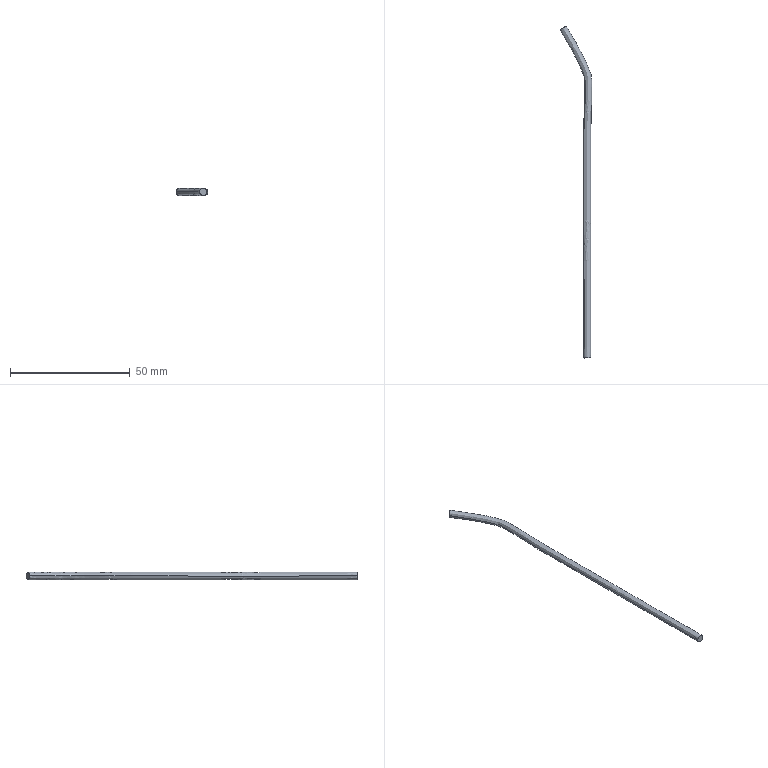Part | NX | features BREP 1 | 1 solid | 4 faces | box 13.379 x 138.71 x 3 mm | volume 977.525 mm3 | plane 2 | spline 2
STEP:
#1=CARTESIAN_POINT('',(-272.402,-33.897,217.465));
#2=VERTEX_POINT('',#1);
#3=CARTESIAN_POINT('',(-269.402,-33.893,217.465));
#4=VERTEX_POINT('',#3);
#5=CARTESIAN_POINT('',(-272.402,-33.897,217.465));
#6=CARTESIAN_POINT('',(-272.402,-33.897,217.819));
#7=CARTESIAN_POINT('',(-272.134,-33.897,218.592));
#8=CARTESIAN_POINT('',(-270.902,-33.895,219.152));
#9=CARTESIAN_POINT('',(-269.67,-33.893,218.592));
#10=CARTESIAN_POINT('',(-269.402,-33.893,217.819));
#11=CARTESIAN_POINT('',(-269.402,-33.893,217.465));
#12=B_SPLINE_CURVE_WITH_KNOTS('',3,(#5,#6,#7,#8,#9,#10,#11),.UNSPECIFIED.,.F.,.F.,(4,1,1,1,4),(0.,0.25,0.5,0.75,1.),.UNSPECIFIED.);
#13=EDGE_CURVE('',#2,#4,#12,.T.);
#14=ORIENTED_EDGE('',*,*,#13,.F.);
#15=CARTESIAN_POINT('',(-269.402,-33.893,217.465));
#16=CARTESIAN_POINT('',(-269.402,-33.893,217.111));
#17=CARTESIAN_POINT('',(-269.67,-33.893,216.338));
#18=CARTESIAN_POINT('',(-270.902,-33.895,215.778));
#19=CARTESIAN_POINT('',(-272.134,-33.897,216.338));
#20=CARTESIAN_POINT('',(-272.402,-33.897,217.111));
#21=CARTESIAN_POINT('',(-272.402,-33.897,217.465));
#22=B_SPLINE_CURVE_WITH_KNOTS('',3,(#15,#16,#17,#18,#19,#20,#21),.UNSPECIFIED.,.F.,.F.,(4,1,1,1,4),(0.,0.25,0.5,0.75,1.),.UNSPECIFIED.);
#23=EDGE_CURVE('',#4,#2,#22,.T.);
#24=ORIENTED_EDGE('',*,*,#23,.F.);
#25=EDGE_LOOP('',(#14,#24));
#26=FACE_BOUND('',#25,.T.);
#27=CARTESIAN_POINT('',(-272.402,-33.897,217.465));
#28=DIRECTION('',(0.001548,-1.,0.000000006));
#29=DIRECTION('',(0.,0.000000006,1.));
#30=AXIS2_PLACEMENT_3D('',#27,#28,#29);
#31=PLANE('',#30);
#32=ADVANCED_FACE('',(#26),#31,.T.);
#33=CARTESIAN_POINT('',(-282.248,103.304,217.465));
#34=VERTEX_POINT('',#33);
#35=CARTESIAN_POINT('',(-282.248,103.304,217.465));
#36=CARTESIAN_POINT('',(-281.519,102.051,217.465));
#37=CARTESIAN_POINT('',(-279.969,99.298,217.465));
#38=CARTESIAN_POINT('',(-277.667,95.455,217.465));
#39=CARTESIAN_POINT('',(-276.,92.4,217.465));
#40=CARTESIAN_POINT('',(-274.733,89.836,217.465));
#41=CARTESIAN_POINT('',(-273.823,87.9,217.465));
#42=CARTESIAN_POINT('',(-272.996,86.076,217.465));
#43=CARTESIAN_POINT('',(-272.458,84.735,217.465));
#44=CARTESIAN_POINT('',(-272.096,83.571,217.465));
#45=CARTESIAN_POINT('',(-271.926,81.973,217.465));
#46=CARTESIAN_POINT('',(-271.863,79.835,217.465));
#47=CARTESIAN_POINT('',(-271.87,77.768,217.465));
#48=CARTESIAN_POINT('',(-271.922,74.793,217.465));
#49=CARTESIAN_POINT('',(-272.002,72.117,217.465));
#50=CARTESIAN_POINT('',(-272.079,69.847,217.465));
#51=CARTESIAN_POINT('',(-272.128,68.501,217.465));
#52=CARTESIAN_POINT('',(-272.168,67.46,217.465));
#53=CARTESIAN_POINT('',(-272.204,66.551,217.465));
#54=CARTESIAN_POINT('',(-272.234,65.828,217.465));
#55=CARTESIAN_POINT('',(-272.257,65.284,217.465));
#56=CARTESIAN_POINT('',(-272.284,64.656,217.465));
#57=CARTESIAN_POINT('',(-272.337,63.497,217.465));
#58=CARTESIAN_POINT('',(-272.394,62.293,217.465));
#59=CARTESIAN_POINT('',(-272.435,61.624,217.465));
#60=CARTESIAN_POINT('',(-272.462,61.03,217.465));
#61=CARTESIAN_POINT('',(-272.465,60.237,217.465));
#62=CARTESIAN_POINT('',(-272.469,59.423,217.465));
#63=CARTESIAN_POINT('',(-272.47,58.473,217.465));
#64=CARTESIAN_POINT('',(-272.471,56.992,217.465));
#65=CARTESIAN_POINT('',(-272.468,54.819,217.465));
#66=CARTESIAN_POINT('',(-272.462,50.705,217.465));
#67=CARTESIAN_POINT('',(-272.455,45.909,217.465));
#68=CARTESIAN_POINT('',(-272.448,41.648,217.465));
#69=CARTESIAN_POINT('',(-272.445,38.887,217.465));
#70=CARTESIAN_POINT('',(-272.443,36.769,217.465));
#71=CARTESIAN_POINT('',(-272.442,34.551,217.465));
#72=CARTESIAN_POINT('',(-272.44,31.729,217.465));
#73=CARTESIAN_POINT('',(-272.439,28.389,217.465));
#74=CARTESIAN_POINT('',(-272.439,24.779,217.465));
#75=CARTESIAN_POINT('',(-272.439,21.455,217.465));
#76=CARTESIAN_POINT('',(-272.439,18.24,217.465));
#77=CARTESIAN_POINT('',(-272.438,13.839,217.465));
#78=CARTESIAN_POINT('',(-272.434,7.607,217.465));
#79=CARTESIAN_POINT('',(-272.425,-1.473,217.465));
#80=CARTESIAN_POINT('',(-272.415,-9.905,217.465));
#81=CARTESIAN_POINT('',(-272.409,-17.422,217.465));
#82=CARTESIAN_POINT('',(-272.409,-25.103,217.465));
#83=CARTESIAN_POINT('',(-272.407,-30.941,217.465));
#84=CARTESIAN_POINT('',(-272.402,-33.897,217.465));
#85=B_SPLINE_CURVE_WITH_KNOTS('',3,(#35,#36,#37,#38,#39,#40,#41,#42,#43,#44,#45,#46,#47,#48,#49,#50,#51,#52,#53,#54,#55,#56,#57,#58,#59,#60,#61,#62,#63,#64,#65,#66,#67,#68,#69,#70,#71,#72,#73,#74,#75,#76,#77,#78,#79,#80,#81,#82,#83,#84),.UNSPECIFIED.,.F.,.F.,(4,1,1,1,1,1,1,1,1,1,1,1,1,1,1,1,1,1,1,1,1,1,1,1,1,1,1,1,1,1,1,1,1,1,1,1,1,1,1,1,1,1,1,1,1,1,1,4),(0.,0.03125,0.0625,0.09375,0.1094,0.125,0.1406,0.1484,0.1562,0.1719,0.1875,0.2031,0.2188,0.25,0.2656,0.2734,0.2812,0.2891,0.293,0.2969,0.3008,0.3047,0.3086,0.3125,0.3164,0.3203,0.3281,0.3359,0.3438,0.3594,0.375,0.3906,0.4062,0.4219,0.4375,0.4531,0.4688,0.5,0.5312,0.5625,0.5938,0.625,0.6875,0.75,0.8125,0.875,0.9375,1.),.UNSPECIFIED.);
#86=EDGE_CURVE('',#34,#2,#85,.T.);
#87=ORIENTED_EDGE('',*,*,#86,.T.);
#88=ORIENTED_EDGE('',*,*,#13,.T.);
#89=CARTESIAN_POINT('',(-279.656,104.812,217.465));
#90=VERTEX_POINT('',#89);
#91=CARTESIAN_POINT('',(-269.402,-33.893,217.465));
#92=CARTESIAN_POINT('',(-269.407,-30.939,217.465));
#93=CARTESIAN_POINT('',(-269.409,-25.105,217.465));
#94=CARTESIAN_POINT('',(-269.409,-17.422,217.465));
#95=CARTESIAN_POINT('',(-269.415,-9.903,217.465));
#96=CARTESIAN_POINT('',(-269.425,-1.469,217.465));
#97=CARTESIAN_POINT('',(-269.434,7.609,217.465));
#98=CARTESIAN_POINT('',(-269.438,13.84,217.465));
#99=CARTESIAN_POINT('',(-269.439,18.241,217.465));
#100=CARTESIAN_POINT('',(-269.439,21.455,217.465));
#101=CARTESIAN_POINT('',(-269.439,24.779,217.465));
#102=CARTESIAN_POINT('',(-269.439,28.39,217.465));
#103=CARTESIAN_POINT('',(-269.44,31.73,217.465));
#104=CARTESIAN_POINT('',(-269.442,34.553,217.465));
#105=CARTESIAN_POINT('',(-269.443,36.772,217.465));
#106=CARTESIAN_POINT('',(-269.445,38.89,217.465));
#107=CARTESIAN_POINT('',(-269.448,41.652,217.465));
#108=CARTESIAN_POINT('',(-269.455,45.913,217.465));
#109=CARTESIAN_POINT('',(-269.462,50.709,217.465));
#110=CARTESIAN_POINT('',(-269.468,54.822,217.465));
#111=CARTESIAN_POINT('',(-269.47,56.995,217.465));
#112=CARTESIAN_POINT('',(-269.47,58.471,217.465));
#113=CARTESIAN_POINT('',(-269.469,59.256,217.465));
#114=CARTESIAN_POINT('',(-269.468,59.891,217.465));
#115=CARTESIAN_POINT('',(-269.464,60.433,217.465));
#116=CARTESIAN_POINT('',(-269.463,60.967,217.465));
#117=CARTESIAN_POINT('',(-269.441,61.414,217.465));
#118=CARTESIAN_POINT('',(-269.396,62.193,217.465));
#119=CARTESIAN_POINT('',(-269.338,63.404,217.465));
#120=CARTESIAN_POINT('',(-269.287,64.532,217.465));
#121=CARTESIAN_POINT('',(-269.26,65.155,217.465));
#122=CARTESIAN_POINT('',(-269.237,65.703,217.465));
#123=CARTESIAN_POINT('',(-269.207,66.431,217.465));
#124=CARTESIAN_POINT('',(-269.17,67.343,217.465));
#125=CARTESIAN_POINT('',(-269.131,68.389,217.465));
#126=CARTESIAN_POINT('',(-269.081,69.742,217.465));
#127=CARTESIAN_POINT('',(-269.004,72.023,217.465));
#128=CARTESIAN_POINT('',(-268.923,74.715,217.465));
#129=CARTESIAN_POINT('',(-268.869,77.729,217.465));
#130=CARTESIAN_POINT('',(-268.866,79.878,217.465));
#131=CARTESIAN_POINT('',(-268.922,82.085,217.465));
#132=CARTESIAN_POINT('',(-269.185,84.586,217.465));
#133=CARTESIAN_POINT('',(-270.095,86.952,217.465));
#134=CARTESIAN_POINT('',(-271.095,89.147,217.465));
#135=CARTESIAN_POINT('',(-272.03,91.139,217.465));
#136=CARTESIAN_POINT('',(-273.338,93.782,217.465));
#137=CARTESIAN_POINT('',(-275.076,96.97,217.465));
#138=CARTESIAN_POINT('',(-277.392,100.831,217.465));
#139=CARTESIAN_POINT('',(-278.898,103.511,217.465));
#140=CARTESIAN_POINT('',(-279.656,104.812,217.465));
#141=B_SPLINE_CURVE_WITH_KNOTS('',3,(#91,#92,#93,#94,#95,#96,#97,#98,#99,#100,#101,#102,#103,#104,#105,#106,#107,#108,#109,#110,#111,#112,#113,#114,#115,#116,#117,#118,#119,#120,#121,#122,#123,#124,#125,#126,#127,#128,#129,#130,#131,#132,#133,#134,#135,#136,#137,#138,#139,#140),.UNSPECIFIED.,.F.,.F.,(4,1,1,1,1,1,1,1,1,1,1,1,1,1,1,1,1,1,1,1,1,1,1,1,1,1,1,1,1,1,1,1,1,1,1,1,1,1,1,1,1,1,1,1,1,1,1,4),(0.,0.0625,0.125,0.1875,0.25,0.3125,0.375,0.4062,0.4375,0.4688,0.5,0.5312,0.5469,0.5625,0.5781,0.5938,0.6094,0.625,0.6406,0.6562,0.6641,0.6719,0.6758,0.6797,0.6836,0.6875,0.6914,0.6953,0.6992,0.7031,0.707,0.7109,0.7188,0.7266,0.7344,0.75,0.7812,0.7969,0.8125,0.8281,0.8438,0.8594,0.875,0.8906,0.9062,0.9375,0.9688,1.),.UNSPECIFIED.);
#142=EDGE_CURVE('',#90,#4,#141,.F.);
#143=ORIENTED_EDGE('',*,*,#142,.F.);
#144=CARTESIAN_POINT('',(-282.248,103.304,217.465));
#145=CARTESIAN_POINT('',(-282.248,103.304,217.819));
#146=CARTESIAN_POINT('',(-282.017,103.438,218.592));
#147=CARTESIAN_POINT('',(-280.952,104.058,219.152));
#148=CARTESIAN_POINT('',(-279.887,104.678,218.592));
#149=CARTESIAN_POINT('',(-279.656,104.812,217.819));
#150=CARTESIAN_POINT('',(-279.656,104.812,217.465));
#151=B_SPLINE_CURVE_WITH_KNOTS('',3,(#144,#145,#146,#147,#148,#149,#150),.UNSPECIFIED.,.F.,.F.,(4,1,1,1,4),(0.,0.25,0.5,0.75,1.),.UNSPECIFIED.);
#152=EDGE_CURVE('',#34,#90,#151,.T.);
#153=ORIENTED_EDGE('',*,*,#152,.F.);
#154=EDGE_LOOP('',(#87,#88,#143,#153));
#155=FACE_BOUND('',#154,.T.);
#156=CARTESIAN_POINT('',(-269.402,-33.893,217.465));
#157=CARTESIAN_POINT('',(-269.402,-33.893,217.819));
#158=CARTESIAN_POINT('',(-269.67,-33.893,218.592));
#159=CARTESIAN_POINT('',(-270.902,-33.895,219.152));
#160=CARTESIAN_POINT('',(-272.134,-33.897,218.592));
#161=CARTESIAN_POINT('',(-272.402,-33.897,217.819));
#162=CARTESIAN_POINT('',(-272.402,-33.897,217.465));
#163=CARTESIAN_POINT('',(-269.404,-32.307,217.465));
#164=CARTESIAN_POINT('',(-269.404,-32.307,217.819));
#165=CARTESIAN_POINT('',(-269.673,-32.307,218.592));
#166=CARTESIAN_POINT('',(-270.904,-32.309,219.152));
#167=CARTESIAN_POINT('',(-272.136,-32.31,218.592));
#168=CARTESIAN_POINT('',(-272.404,-32.31,217.819));
#169=CARTESIAN_POINT('',(-272.404,-32.31,217.465));
#170=CARTESIAN_POINT('',(-269.407,-29.144,217.465));
#171=CARTESIAN_POINT('',(-269.407,-29.144,217.819));
#172=CARTESIAN_POINT('',(-269.675,-29.144,218.592));
#173=CARTESIAN_POINT('',(-270.907,-29.144,219.152));
#174=CARTESIAN_POINT('',(-272.139,-29.144,218.592));
#175=CARTESIAN_POINT('',(-272.407,-29.145,217.819));
#176=CARTESIAN_POINT('',(-272.407,-29.145,217.465));
#177=CARTESIAN_POINT('',(-269.409,-23.132,217.465));
#178=CARTESIAN_POINT('',(-269.409,-23.132,217.819));
#179=CARTESIAN_POINT('',(-269.677,-23.132,218.592));
#180=CARTESIAN_POINT('',(-270.909,-23.132,219.152));
#181=CARTESIAN_POINT('',(-272.14,-23.131,218.592));
#182=CARTESIAN_POINT('',(-272.409,-23.131,217.819));
#183=CARTESIAN_POINT('',(-272.409,-23.131,217.465));
#184=CARTESIAN_POINT('',(-269.409,-16.333,217.465));
#185=CARTESIAN_POINT('',(-269.409,-16.333,217.819));
#186=CARTESIAN_POINT('',(-269.678,-16.333,218.592));
#187=CARTESIAN_POINT('',(-270.909,-16.333,219.152));
#188=CARTESIAN_POINT('',(-272.141,-16.333,218.592));
#189=CARTESIAN_POINT('',(-272.409,-16.333,217.819));
#190=CARTESIAN_POINT('',(-272.409,-16.333,217.465));
#191=CARTESIAN_POINT('',(-269.416,-9.531,217.465));
#192=CARTESIAN_POINT('',(-269.416,-9.531,217.819));
#193=CARTESIAN_POINT('',(-269.684,-9.531,218.592));
#194=CARTESIAN_POINT('',(-270.916,-9.532,219.152));
#195=CARTESIAN_POINT('',(-272.147,-9.533,218.592));
#196=CARTESIAN_POINT('',(-272.416,-9.534,217.819));
#197=CARTESIAN_POINT('',(-272.416,-9.534,217.465));
#198=CARTESIAN_POINT('',(-269.422,-3.52,217.465));
#199=CARTESIAN_POINT('',(-269.422,-3.52,217.819));
#200=CARTESIAN_POINT('',(-269.691,-3.521,218.592));
#201=CARTESIAN_POINT('',(-270.922,-3.522,219.152));
#202=CARTESIAN_POINT('',(-272.154,-3.523,218.592));
#203=CARTESIAN_POINT('',(-272.422,-3.524,217.819));
#204=CARTESIAN_POINT('',(-272.422,-3.524,217.465));
#205=CARTESIAN_POINT('',(-269.428,1.443,217.465));
#206=CARTESIAN_POINT('',(-269.428,1.443,217.819));
#207=CARTESIAN_POINT('',(-269.696,1.443,218.592));
#208=CARTESIAN_POINT('',(-270.928,1.441,219.152));
#209=CARTESIAN_POINT('',(-272.16,1.44,218.592));
#210=CARTESIAN_POINT('',(-272.428,1.44,217.819));
#211=CARTESIAN_POINT('',(-272.428,1.44,217.465));
#212=CARTESIAN_POINT('',(-269.433,6.608,217.465));
#213=CARTESIAN_POINT('',(-269.433,6.608,217.819));
#214=CARTESIAN_POINT('',(-269.701,6.608,218.592));
#215=CARTESIAN_POINT('',(-270.933,6.607,219.152));
#216=CARTESIAN_POINT('',(-272.165,6.606,218.592));
#217=CARTESIAN_POINT('',(-272.433,6.605,217.819));
#218=CARTESIAN_POINT('',(-272.433,6.605,217.465));
#219=CARTESIAN_POINT('',(-269.437,11.462,217.465));
#220=CARTESIAN_POINT('',(-269.437,11.462,217.819));
#221=CARTESIAN_POINT('',(-269.705,11.462,218.592));
#222=CARTESIAN_POINT('',(-270.937,11.461,219.152));
#223=CARTESIAN_POINT('',(-272.168,11.46,218.592));
#224=CARTESIAN_POINT('',(-272.437,11.46,217.819));
#225=CARTESIAN_POINT('',(-272.437,11.46,217.465));
#226=CARTESIAN_POINT('',(-269.438,15.751,217.465));
#227=CARTESIAN_POINT('',(-269.438,15.751,217.819));
#228=CARTESIAN_POINT('',(-269.707,15.751,218.592));
#229=CARTESIAN_POINT('',(-270.938,15.75,219.152));
#230=CARTESIAN_POINT('',(-272.17,15.75,218.592));
#231=CARTESIAN_POINT('',(-272.438,15.75,217.819));
#232=CARTESIAN_POINT('',(-272.438,15.75,217.465));
#233=CARTESIAN_POINT('',(-269.439,19.687,217.465));
#234=CARTESIAN_POINT('',(-269.439,19.687,217.819));
#235=CARTESIAN_POINT('',(-269.707,19.687,218.592));
#236=CARTESIAN_POINT('',(-270.939,19.687,219.152));
#237=CARTESIAN_POINT('',(-272.17,19.687,218.592));
#238=CARTESIAN_POINT('',(-272.439,19.687,217.819));
#239=CARTESIAN_POINT('',(-272.439,19.687,217.465));
#240=CARTESIAN_POINT('',(-269.439,23.624,217.465));
#241=CARTESIAN_POINT('',(-269.439,23.624,217.819));
#242=CARTESIAN_POINT('',(-269.707,23.624,218.592));
#243=CARTESIAN_POINT('',(-270.939,23.625,219.152));
#244=CARTESIAN_POINT('',(-272.17,23.625,218.592));
#245=CARTESIAN_POINT('',(-272.439,23.625,217.819));
#246=CARTESIAN_POINT('',(-272.439,23.625,217.465));
#247=CARTESIAN_POINT('',(-269.439,27.912,217.465));
#248=CARTESIAN_POINT('',(-269.439,27.912,217.819));
#249=CARTESIAN_POINT('',(-269.707,27.912,218.592));
#250=CARTESIAN_POINT('',(-270.939,27.911,219.152));
#251=CARTESIAN_POINT('',(-272.17,27.911,218.592));
#252=CARTESIAN_POINT('',(-272.439,27.911,217.819));
#253=CARTESIAN_POINT('',(-272.439,27.911,217.465));
#254=CARTESIAN_POINT('',(-269.44,32.775,217.465));
#255=CARTESIAN_POINT('',(-269.44,32.775,217.819));
#256=CARTESIAN_POINT('',(-269.709,32.775,218.592));
#257=CARTESIAN_POINT('',(-270.94,32.775,219.152));
#258=CARTESIAN_POINT('',(-272.172,32.774,218.592));
#259=CARTESIAN_POINT('',(-272.44,32.774,217.819));
#260=CARTESIAN_POINT('',(-272.44,32.774,217.465));
#261=CARTESIAN_POINT('',(-269.443,36.852,217.465));
#262=CARTESIAN_POINT('',(-269.443,36.852,217.819));
#263=CARTESIAN_POINT('',(-269.711,36.852,218.592));
#264=CARTESIAN_POINT('',(-270.943,36.851,219.152));
#265=CARTESIAN_POINT('',(-272.175,36.85,218.592));
#266=CARTESIAN_POINT('',(-272.443,36.85,217.819));
#267=CARTESIAN_POINT('',(-272.443,36.85,217.465));
#268=CARTESIAN_POINT('',(-269.446,39.72,217.465));
#269=CARTESIAN_POINT('',(-269.446,39.72,217.819));
#270=CARTESIAN_POINT('',(-269.714,39.72,218.592));
#271=CARTESIAN_POINT('',(-270.946,39.719,219.152));
#272=CARTESIAN_POINT('',(-272.178,39.717,218.592));
#273=CARTESIAN_POINT('',(-272.446,39.717,217.819));
#274=CARTESIAN_POINT('',(-272.446,39.717,217.465));
#275=CARTESIAN_POINT('',(-269.449,41.909,217.465));
#276=CARTESIAN_POINT('',(-269.449,41.909,217.819));
#277=CARTESIAN_POINT('',(-269.717,41.908,218.592));
#278=CARTESIAN_POINT('',(-270.949,41.907,219.152));
#279=CARTESIAN_POINT('',(-272.181,41.906,218.592));
#280=CARTESIAN_POINT('',(-272.449,41.905,217.819));
#281=CARTESIAN_POINT('',(-272.449,41.905,217.465));
#282=CARTESIAN_POINT('',(-269.453,44.762,217.465));
#283=CARTESIAN_POINT('',(-269.453,44.762,217.819));
#284=CARTESIAN_POINT('',(-269.721,44.762,218.592));
#285=CARTESIAN_POINT('',(-270.953,44.76,219.152));
#286=CARTESIAN_POINT('',(-272.185,44.759,218.592));
#287=CARTESIAN_POINT('',(-272.453,44.759,217.819));
#288=CARTESIAN_POINT('',(-272.453,44.759,217.465));
#289=CARTESIAN_POINT('',(-269.458,48.03,217.465));
#290=CARTESIAN_POINT('',(-269.458,48.03,217.819));
#291=CARTESIAN_POINT('',(-269.726,48.03,218.592));
#292=CARTESIAN_POINT('',(-270.958,48.028,219.152));
#293=CARTESIAN_POINT('',(-272.189,48.027,218.592));
#294=CARTESIAN_POINT('',(-272.458,48.027,217.819));
#295=CARTESIAN_POINT('',(-272.458,48.027,217.465));
#296=CARTESIAN_POINT('',(-269.463,51.297,217.465));
#297=CARTESIAN_POINT('',(-269.463,51.297,217.819));
#298=CARTESIAN_POINT('',(-269.731,51.297,218.592));
#299=CARTESIAN_POINT('',(-270.963,51.296,219.152));
#300=CARTESIAN_POINT('',(-272.195,51.294,218.592));
#301=CARTESIAN_POINT('',(-272.463,51.294,217.819));
#302=CARTESIAN_POINT('',(-272.463,51.294,217.465));
#303=CARTESIAN_POINT('',(-269.467,54.151,217.465));
#304=CARTESIAN_POINT('',(-269.467,54.151,217.819));
#305=CARTESIAN_POINT('',(-269.735,54.151,218.592));
#306=CARTESIAN_POINT('',(-270.967,54.15,219.152));
#307=CARTESIAN_POINT('',(-272.199,54.149,218.592));
#308=CARTESIAN_POINT('',(-272.467,54.148,217.819));
#309=CARTESIAN_POINT('',(-272.467,54.148,217.465));
#310=CARTESIAN_POINT('',(-269.47,56.336,217.465));
#311=CARTESIAN_POINT('',(-269.47,56.336,217.819));
#312=CARTESIAN_POINT('',(-269.738,56.336,218.592));
#313=CARTESIAN_POINT('',(-270.97,56.335,219.152));
#314=CARTESIAN_POINT('',(-272.202,56.334,218.592));
#315=CARTESIAN_POINT('',(-272.47,56.334,217.819));
#316=CARTESIAN_POINT('',(-272.47,56.334,217.465));
#317=CARTESIAN_POINT('',(-269.47,57.645,217.465));
#318=CARTESIAN_POINT('',(-269.47,57.645,217.819));
#319=CARTESIAN_POINT('',(-269.739,57.645,218.592));
#320=CARTESIAN_POINT('',(-270.97,57.645,219.152));
#321=CARTESIAN_POINT('',(-272.202,57.644,218.592));
#322=CARTESIAN_POINT('',(-272.47,57.644,217.819));
#323=CARTESIAN_POINT('',(-272.47,57.644,217.465));
#324=CARTESIAN_POINT('',(-269.47,58.64,217.465));
#325=CARTESIAN_POINT('',(-269.47,58.64,217.819));
#326=CARTESIAN_POINT('',(-269.738,58.64,218.592));
#327=CARTESIAN_POINT('',(-270.97,58.642,219.152));
#328=CARTESIAN_POINT('',(-272.202,58.643,218.592));
#329=CARTESIAN_POINT('',(-272.47,58.644,217.819));
#330=CARTESIAN_POINT('',(-272.47,58.644,217.465));
#331=CARTESIAN_POINT('',(-269.469,59.264,217.465));
#332=CARTESIAN_POINT('',(-269.469,59.264,217.819));
#333=CARTESIAN_POINT('',(-269.737,59.265,218.592));
#334=CARTESIAN_POINT('',(-270.969,59.269,219.152));
#335=CARTESIAN_POINT('',(-272.2,59.274,218.592));
#336=CARTESIAN_POINT('',(-272.469,59.275,217.819));
#337=CARTESIAN_POINT('',(-272.469,59.275,217.465));
#338=CARTESIAN_POINT('',(-269.468,59.888,217.465));
#339=CARTESIAN_POINT('',(-269.468,59.888,217.819));
#340=CARTESIAN_POINT('',(-269.736,59.89,218.592));
#341=CARTESIAN_POINT('',(-270.968,59.897,219.152));
#342=CARTESIAN_POINT('',(-272.199,59.905,218.592));
#343=CARTESIAN_POINT('',(-272.468,59.907,217.819));
#344=CARTESIAN_POINT('',(-272.468,59.907,217.465));
#345=CARTESIAN_POINT('',(-269.464,60.504,217.465));
#346=CARTESIAN_POINT('',(-269.464,60.504,217.819));
#347=CARTESIAN_POINT('',(-269.732,60.504,218.592));
#348=CARTESIAN_POINT('',(-270.964,60.506,219.152));
#349=CARTESIAN_POINT('',(-272.196,60.507,218.592));
#350=CARTESIAN_POINT('',(-272.464,60.507,217.819));
#351=CARTESIAN_POINT('',(-272.464,60.507,217.465));
#352=CARTESIAN_POINT('',(-269.461,60.971,217.465));
#353=CARTESIAN_POINT('',(-269.461,60.971,217.819));
#354=CARTESIAN_POINT('',(-269.729,60.977,218.592));
#355=CARTESIAN_POINT('',(-270.961,61.006,219.152));
#356=CARTESIAN_POINT('',(-272.192,61.034,218.592));
#357=CARTESIAN_POINT('',(-272.46,61.041,217.819));
#358=CARTESIAN_POINT('',(-272.46,61.041,217.465));
#359=CARTESIAN_POINT('',(-269.445,61.346,217.465));
#360=CARTESIAN_POINT('',(-269.445,61.346,217.819));
#361=CARTESIAN_POINT('',(-269.713,61.365,218.592));
#362=CARTESIAN_POINT('',(-270.942,61.449,219.152));
#363=CARTESIAN_POINT('',(-272.171,61.532,218.592));
#364=CARTESIAN_POINT('',(-272.439,61.551,217.819));
#365=CARTESIAN_POINT('',(-272.439,61.551,217.465));
#366=CARTESIAN_POINT('',(-269.407,61.976,217.465));
#367=CARTESIAN_POINT('',(-269.407,61.976,217.819));
#368=CARTESIAN_POINT('',(-269.675,61.986,218.592));
#369=CARTESIAN_POINT('',(-270.906,62.034,219.152));
#370=CARTESIAN_POINT('',(-272.137,62.081,218.592));
#371=CARTESIAN_POINT('',(-272.405,62.092,217.819));
#372=CARTESIAN_POINT('',(-272.405,62.092,217.465));
#373=CARTESIAN_POINT('',(-269.344,63.273,217.465));
#374=CARTESIAN_POINT('',(-269.344,63.273,217.819));
#375=CARTESIAN_POINT('',(-269.612,63.281,218.592));
#376=CARTESIAN_POINT('',(-270.843,63.317,219.152));
#377=CARTESIAN_POINT('',(-272.075,63.353,218.592));
#378=CARTESIAN_POINT('',(-272.343,63.361,217.819));
#379=CARTESIAN_POINT('',(-272.343,63.361,217.465));
#380=CARTESIAN_POINT('',(-269.286,64.54,217.465));
#381=CARTESIAN_POINT('',(-269.286,64.54,217.819));
#382=CARTESIAN_POINT('',(-269.554,64.552,218.592));
#383=CARTESIAN_POINT('',(-270.785,64.603,219.152));
#384=CARTESIAN_POINT('',(-272.016,64.654,218.592));
#385=CARTESIAN_POINT('',(-272.284,64.665,217.819));
#386=CARTESIAN_POINT('',(-272.284,64.665,217.465));
#387=CARTESIAN_POINT('',(-269.255,65.265,217.465));
#388=CARTESIAN_POINT('',(-269.255,65.265,217.819));
#389=CARTESIAN_POINT('',(-269.523,65.277,218.592));
#390=CARTESIAN_POINT('',(-270.754,65.33,219.152));
#391=CARTESIAN_POINT('',(-271.984,65.383,218.592));
#392=CARTESIAN_POINT('',(-272.252,65.395,217.819));
#393=CARTESIAN_POINT('',(-272.252,65.395,217.465));
#394=CARTESIAN_POINT('',(-269.225,65.969,217.465));
#395=CARTESIAN_POINT('',(-269.225,65.969,217.819));
#396=CARTESIAN_POINT('',(-269.494,65.98,218.592));
#397=CARTESIAN_POINT('',(-270.724,66.031,219.152));
#398=CARTESIAN_POINT('',(-271.955,66.081,218.592));
#399=CARTESIAN_POINT('',(-272.223,66.092,217.819));
#400=CARTESIAN_POINT('',(-272.223,66.092,217.465));
#401=CARTESIAN_POINT('',(-269.184,67.005,217.465));
#402=CARTESIAN_POINT('',(-269.184,67.005,217.819));
#403=CARTESIAN_POINT('',(-269.452,67.016,218.592));
#404=CARTESIAN_POINT('',(-270.682,67.065,219.152));
#405=CARTESIAN_POINT('',(-271.913,67.113,218.592));
#406=CARTESIAN_POINT('',(-272.181,67.124,217.819));
#407=CARTESIAN_POINT('',(-272.181,67.124,217.465));
#408=CARTESIAN_POINT('',(-269.116,68.749,217.465));
#409=CARTESIAN_POINT('',(-269.116,68.749,217.819));
#410=CARTESIAN_POINT('',(-269.384,68.759,218.592));
#411=CARTESIAN_POINT('',(-270.615,68.804,219.152));
#412=CARTESIAN_POINT('',(-271.846,68.848,218.592));
#413=CARTESIAN_POINT('',(-272.114,68.858,217.819));
#414=CARTESIAN_POINT('',(-272.114,68.858,217.465));
#415=CARTESIAN_POINT('',(-269.035,71.062,217.465));
#416=CARTESIAN_POINT('',(-269.035,71.062,217.819));
#417=CARTESIAN_POINT('',(-269.303,71.07,218.592));
#418=CARTESIAN_POINT('',(-270.534,71.111,219.152));
#419=CARTESIAN_POINT('',(-271.765,71.152,218.592));
#420=CARTESIAN_POINT('',(-272.033,71.16,217.819));
#421=CARTESIAN_POINT('',(-272.033,71.16,217.465));
#422=CARTESIAN_POINT('',(-268.95,73.826,217.465));
#423=CARTESIAN_POINT('',(-268.95,73.826,217.819));
#424=CARTESIAN_POINT('',(-269.218,73.834,218.592));
#425=CARTESIAN_POINT('',(-270.449,73.868,219.152));
#426=CARTESIAN_POINT('',(-271.681,73.902,218.592));
#427=CARTESIAN_POINT('',(-271.949,73.909,217.819));
#428=CARTESIAN_POINT('',(-271.949,73.909,217.465));
#429=CARTESIAN_POINT('',(-268.891,76.327,217.465));
#430=CARTESIAN_POINT('',(-268.891,76.327,217.819));
#431=CARTESIAN_POINT('',(-269.159,76.333,218.592));
#432=CARTESIAN_POINT('',(-270.39,76.357,219.152));
#433=CARTESIAN_POINT('',(-271.622,76.381,218.592));
#434=CARTESIAN_POINT('',(-271.89,76.387,217.819));
#435=CARTESIAN_POINT('',(-271.89,76.387,217.465));
#436=CARTESIAN_POINT('',(-268.869,78.25,217.465));
#437=CARTESIAN_POINT('',(-268.869,78.25,217.819));
#438=CARTESIAN_POINT('',(-269.137,78.252,218.592));
#439=CARTESIAN_POINT('',(-270.369,78.26,219.152));
#440=CARTESIAN_POINT('',(-271.6,78.268,218.592));
#441=CARTESIAN_POINT('',(-271.869,78.269,217.819));
#442=CARTESIAN_POINT('',(-271.869,78.269,217.465));
#443=CARTESIAN_POINT('',(-268.869,79.511,217.465));
#444=CARTESIAN_POINT('',(-268.869,79.511,217.819));
#445=CARTESIAN_POINT('',(-269.137,79.509,218.592));
#446=CARTESIAN_POINT('',(-270.368,79.5,219.152));
#447=CARTESIAN_POINT('',(-271.6,79.491,218.592));
#448=CARTESIAN_POINT('',(-271.868,79.489,217.819));
#449=CARTESIAN_POINT('',(-271.868,79.489,217.465));
#450=CARTESIAN_POINT('',(-268.888,80.782,217.465));
#451=CARTESIAN_POINT('',(-268.888,80.782,217.819));
#452=CARTESIAN_POINT('',(-269.156,80.774,218.592));
#453=CARTESIAN_POINT('',(-270.388,80.74,219.152));
#454=CARTESIAN_POINT('',(-271.619,80.706,218.592));
#455=CARTESIAN_POINT('',(-271.887,80.699,217.819));
#456=CARTESIAN_POINT('',(-271.887,80.699,217.465));
#457=CARTESIAN_POINT('',(-268.948,82.143,217.465));
#458=CARTESIAN_POINT('',(-268.948,82.143,217.819));
#459=CARTESIAN_POINT('',(-269.215,82.127,218.592));
#460=CARTESIAN_POINT('',(-270.445,82.054,219.152));
#461=CARTESIAN_POINT('',(-271.674,81.981,218.592));
#462=CARTESIAN_POINT('',(-271.942,81.965,217.819));
#463=CARTESIAN_POINT('',(-271.942,81.965,217.465));
#464=CARTESIAN_POINT('',(-269.068,83.589,217.465));
#465=CARTESIAN_POINT('',(-269.068,83.589,217.819));
#466=CARTESIAN_POINT('',(-269.335,83.552,218.592));
#467=CARTESIAN_POINT('',(-270.559,83.385,219.152));
#468=CARTESIAN_POINT('',(-271.783,83.218,218.592));
#469=CARTESIAN_POINT('',(-272.05,83.182,217.819));
#470=CARTESIAN_POINT('',(-272.05,83.182,217.465));
#471=CARTESIAN_POINT('',(-269.389,85.055,217.465));
#472=CARTESIAN_POINT('',(-269.389,85.055,217.819));
#473=CARTESIAN_POINT('',(-269.647,84.977,218.592));
#474=CARTESIAN_POINT('',(-270.829,84.619,219.152));
#475=CARTESIAN_POINT('',(-272.011,84.26,218.592));
#476=CARTESIAN_POINT('',(-272.269,84.182,217.819));
#477=CARTESIAN_POINT('',(-272.269,84.182,217.465));
#478=CARTESIAN_POINT('',(-269.85,86.313,217.465));
#479=CARTESIAN_POINT('',(-269.85,86.313,217.819));
#480=CARTESIAN_POINT('',(-270.098,86.212,218.592));
#481=CARTESIAN_POINT('',(-271.24,85.749,219.152));
#482=CARTESIAN_POINT('',(-272.382,85.286,218.592));
#483=CARTESIAN_POINT('',(-272.631,85.185,217.819));
#484=CARTESIAN_POINT('',(-272.631,85.185,217.465));
#485=CARTESIAN_POINT('',(-270.342,87.473,217.465));
#486=CARTESIAN_POINT('',(-270.342,87.473,217.819));
#487=CARTESIAN_POINT('',(-270.587,87.364,218.592));
#488=CARTESIAN_POINT('',(-271.712,86.862,219.152));
#489=CARTESIAN_POINT('',(-272.837,86.361,218.592));
#490=CARTESIAN_POINT('',(-273.082,86.252,217.819));
#491=CARTESIAN_POINT('',(-273.082,86.252,217.465));
#492=CARTESIAN_POINT('',(-270.844,88.591,217.465));
#493=CARTESIAN_POINT('',(-270.844,88.591,217.819));
#494=CARTESIAN_POINT('',(-271.088,88.48,218.592));
#495=CARTESIAN_POINT('',(-272.208,87.969,219.152));
#496=CARTESIAN_POINT('',(-273.329,87.457,218.592));
#497=CARTESIAN_POINT('',(-273.573,87.346,217.819));
#498=CARTESIAN_POINT('',(-273.573,87.346,217.465));
#499=CARTESIAN_POINT('',(-271.865,90.809,217.465));
#500=CARTESIAN_POINT('',(-271.865,90.809,217.819));
#501=CARTESIAN_POINT('',(-272.107,90.694,218.592));
#502=CARTESIAN_POINT('',(-273.22,90.165,219.152));
#503=CARTESIAN_POINT('',(-274.332,89.636,218.592));
#504=CARTESIAN_POINT('',(-274.575,89.52,217.819));
#505=CARTESIAN_POINT('',(-274.575,89.52,217.465));
#506=CARTESIAN_POINT('',(-273.108,93.352,217.465));
#507=CARTESIAN_POINT('',(-273.108,93.352,217.819));
#508=CARTESIAN_POINT('',(-273.347,93.23,218.592));
#509=CARTESIAN_POINT('',(-274.443,92.668,219.152));
#510=CARTESIAN_POINT('',(-275.539,92.106,218.592));
#511=CARTESIAN_POINT('',(-275.778,91.983,217.819));
#512=CARTESIAN_POINT('',(-275.778,91.983,217.465));
#513=CARTESIAN_POINT('',(-274.668,96.211,217.465));
#514=CARTESIAN_POINT('',(-274.668,96.211,217.819));
#515=CARTESIAN_POINT('',(-274.901,96.079,218.592));
#516=CARTESIAN_POINT('',(-275.974,95.473,219.152));
#517=CARTESIAN_POINT('',(-277.046,94.867,218.592));
#518=CARTESIAN_POINT('',(-277.28,94.735,217.819));
#519=CARTESIAN_POINT('',(-277.28,94.735,217.465));
#520=CARTESIAN_POINT('',(-275.808,98.18,217.465));
#521=CARTESIAN_POINT('',(-275.808,98.18,217.819));
#522=CARTESIAN_POINT('',(-276.039,98.044,218.592));
#523=CARTESIAN_POINT('',(-277.101,97.419,219.152));
#524=CARTESIAN_POINT('',(-278.163,96.795,218.592));
#525=CARTESIAN_POINT('',(-278.394,96.659,217.819));
#526=CARTESIAN_POINT('',(-278.394,96.659,217.465));
#527=CARTESIAN_POINT('',(-276.849,99.943,217.465));
#528=CARTESIAN_POINT('',(-276.849,99.943,217.819));
#529=CARTESIAN_POINT('',(-277.08,99.807,218.592));
#530=CARTESIAN_POINT('',(-278.141,99.182,219.152));
#531=CARTESIAN_POINT('',(-279.202,98.556,218.592));
#532=CARTESIAN_POINT('',(-279.433,98.42,217.819));
#533=CARTESIAN_POINT('',(-279.433,98.42,217.465));
#534=CARTESIAN_POINT('',(-277.804,101.577,217.465));
#535=CARTESIAN_POINT('',(-277.804,101.577,217.819));
#536=CARTESIAN_POINT('',(-278.036,101.443,218.592));
#537=CARTESIAN_POINT('',(-279.101,100.825,219.152));
#538=CARTESIAN_POINT('',(-280.166,100.207,218.592));
#539=CARTESIAN_POINT('',(-280.399,100.073,217.819));
#540=CARTESIAN_POINT('',(-280.399,100.073,217.465));
#541=CARTESIAN_POINT('',(-278.742,103.218,217.465));
#542=CARTESIAN_POINT('',(-278.742,103.218,217.819));
#543=CARTESIAN_POINT('',(-278.976,103.085,218.592));
#544=CARTESIAN_POINT('',(-280.046,102.477,219.152));
#545=CARTESIAN_POINT('',(-281.117,101.868,218.592));
#546=CARTESIAN_POINT('',(-281.35,101.736,217.819));
#547=CARTESIAN_POINT('',(-281.35,101.736,217.465));
#548=CARTESIAN_POINT('',(-279.345,104.279,217.465));
#549=CARTESIAN_POINT('',(-279.345,104.279,217.819));
#550=CARTESIAN_POINT('',(-279.578,104.146,218.592));
#551=CARTESIAN_POINT('',(-280.648,103.535,219.152));
#552=CARTESIAN_POINT('',(-281.717,102.923,218.592));
#553=CARTESIAN_POINT('',(-281.95,102.79,217.819));
#554=CARTESIAN_POINT('',(-281.95,102.79,217.465));
#555=CARTESIAN_POINT('',(-279.656,104.812,217.465));
#556=CARTESIAN_POINT('',(-279.656,104.812,217.819));
#557=CARTESIAN_POINT('',(-279.887,104.678,218.592));
#558=CARTESIAN_POINT('',(-280.952,104.058,219.152));
#559=CARTESIAN_POINT('',(-282.017,103.438,218.592));
#560=CARTESIAN_POINT('',(-282.248,103.304,217.819));
#561=CARTESIAN_POINT('',(-282.248,103.304,217.465));
#562=B_SPLINE_SURFACE_WITH_KNOTS('',3,3,((#156,#157,#158,#159,#160,#161,#162),(#163,#164,#165,#166,#167,#168,#169),(#170,#171,#172,#173,#174,#175,#176),(#177,#178,#179,#180,#181,#182,#183),(#184,#185,#186,#187,#188,#189,#190),(#191,#192,#193,#194,#195,#196,#197),(#198,#199,#200,#201,#202,#203,#204),(#205,#206,#207,#208,#209,#210,#211),(#212,#213,#214,#215,#216,#217,#218),(#219,#220,#221,#222,#223,#224,#225),(#226,#227,#228,#229,#230,#231,#232),(#233,#234,#235,#236,#237,#238,#239),(#240,#241,#242,#243,#244,#245,#246),(#247,#248,#249,#250,#251,#252,#253),(#254,#255,#256,#257,#258,#259,#260),(#261,#262,#263,#264,#265,#266,#267),(#268,#269,#270,#271,#272,#273,#274),(#275,#276,#277,#278,#279,#280,#281),(#282,#283,#284,#285,#286,#287,#288),(#289,#290,#291,#292,#293,#294,#295),(#296,#297,#298,#299,#300,#301,#302),(#303,#304,#305,#306,#307,#308,#309),(#310,#311,#312,#313,#314,#315,#316),(#317,#318,#319,#320,#321,#322,#323),(#324,#325,#326,#327,#328,#329,#330),(#331,#332,#333,#334,#335,#336,#337),(#338,#339,#340,#341,#342,#343,#344),(#345,#346,#347,#348,#349,#350,#351),(#352,#353,#354,#355,#356,#357,#358),(#359,#360,#361,#362,#363,#364,#365),(#366,#367,#368,#369,#370,#371,#372),(#373,#374,#375,#376,#377,#378,#379),(#380,#381,#382,#383,#384,#385,#386),(#387,#388,#389,#390,#391,#392,#393),(#394,#395,#396,#397,#398,#399,#400),(#401,#402,#403,#404,#405,#406,#407),(#408,#409,#410,#411,#412,#413,#414),(#415,#416,#417,#418,#419,#420,#421),(#422,#423,#424,#425,#426,#427,#428),(#429,#430,#431,#432,#433,#434,#435),(#436,#437,#438,#439,#440,#441,#442),(#443,#444,#445,#446,#447,#448,#449),(#450,#451,#452,#453,#454,#455,#456),(#457,#458,#459,#460,#461,#462,#463),(#464,#465,#466,#467,#468,#469,#470),(#471,#472,#473,#474,#475,#476,#477),(#478,#479,#480,#481,#482,#483,#484),(#485,#486,#487,#488,#489,#490,#491),(#492,#493,#494,#495,#496,#497,#498),(#499,#500,#501,#502,#503,#504,#505),(#506,#507,#508,#509,#510,#511,#512),(#513,#514,#515,#516,#517,#518,#519),(#520,#521,#522,#523,#524,#525,#526),(#527,#528,#529,#530,#531,#532,#533),(#534,#535,#536,#537,#538,#539,#540),(#541,#542,#543,#544,#545,#546,#547),(#548,#549,#550,#551,#552,#553,#554),(#555,#556,#557,#558,#559,#560,#561)),.UNSPECIFIED.,.F.,.F.,.F.,(4,1,1,1,1,1,1,1,1,1,1,1,1,1,1,1,1,1,1,1,1,1,1,1,1,1,1,1,1,1,1,1,1,1,1,1,1,1,1,1,1,1,1,1,1,1,1,1,1,1,1,1,1,1,1,4),(4,1,1,1,4),(0.009617,0.04252,0.07542,0.1412,0.207,0.2399,0.2728,0.3101,0.3473,0.3846,0.4219,0.4591,0.4964,0.5337,0.5709,0.5817,0.5925,0.6033,0.614,0.6248,0.6356,0.6464,0.6572,0.6623,0.6674,0.6725,0.6776,0.6802,0.6828,0.687,0.6912,0.6954,0.6996,0.705,0.7104,0.7212,0.7427,0.7643,0.7859,0.7949,0.8039,0.8128,0.8218,0.8312,0.8407,0.8484,0.8562,0.8639,0.8717,0.9059,0.9231,0.9402,0.9528,0.9653,0.9779,0.9904),(0.02118,0.2607,0.5002,0.7397,0.9792),.UNSPECIFIED.);
#563=ADVANCED_FACE('',(#155),#562,.T.);
#564=ORIENTED_EDGE('',*,*,#142,.T.);
#565=ORIENTED_EDGE('',*,*,#23,.T.);
#566=ORIENTED_EDGE('',*,*,#86,.F.);
#567=CARTESIAN_POINT('',(-279.656,104.812,217.465));
#568=CARTESIAN_POINT('',(-279.656,104.812,217.111));
#569=CARTESIAN_POINT('',(-279.887,104.678,216.338));
#570=CARTESIAN_POINT('',(-280.952,104.058,215.778));
#571=CARTESIAN_POINT('',(-282.017,103.438,216.338));
#572=CARTESIAN_POINT('',(-282.248,103.304,217.111));
#573=CARTESIAN_POINT('',(-282.248,103.304,217.465));
#574=B_SPLINE_CURVE_WITH_KNOTS('',3,(#567,#568,#569,#570,#571,#572,#573),.UNSPECIFIED.,.F.,.F.,(4,1,1,1,4),(0.,0.25,0.5,0.75,1.),.UNSPECIFIED.);
#575=EDGE_CURVE('',#90,#34,#574,.T.);
#576=ORIENTED_EDGE('',*,*,#575,.F.);
#577=EDGE_LOOP('',(#564,#565,#566,#576));
#578=FACE_BOUND('',#577,.T.);
#579=CARTESIAN_POINT('',(-272.402,-33.897,217.465));
#580=CARTESIAN_POINT('',(-272.402,-33.897,217.111));
#581=CARTESIAN_POINT('',(-272.134,-33.897,216.338));
#582=CARTESIAN_POINT('',(-270.902,-33.895,215.778));
#583=CARTESIAN_POINT('',(-269.67,-33.893,216.338));
#584=CARTESIAN_POINT('',(-269.402,-33.893,217.111));
#585=CARTESIAN_POINT('',(-269.402,-33.893,217.465));
#586=CARTESIAN_POINT('',(-272.404,-32.31,217.465));
#587=CARTESIAN_POINT('',(-272.404,-32.31,217.111));
#588=CARTESIAN_POINT('',(-272.136,-32.31,216.338));
#589=CARTESIAN_POINT('',(-270.904,-32.309,215.778));
#590=CARTESIAN_POINT('',(-269.673,-32.307,216.338));
#591=CARTESIAN_POINT('',(-269.404,-32.307,217.111));
#592=CARTESIAN_POINT('',(-269.404,-32.307,217.465));
#593=CARTESIAN_POINT('',(-272.407,-29.145,217.465));
#594=CARTESIAN_POINT('',(-272.407,-29.145,217.111));
#595=CARTESIAN_POINT('',(-272.139,-29.144,216.338));
#596=CARTESIAN_POINT('',(-270.907,-29.144,215.778));
#597=CARTESIAN_POINT('',(-269.675,-29.144,216.338));
#598=CARTESIAN_POINT('',(-269.407,-29.144,217.111));
#599=CARTESIAN_POINT('',(-269.407,-29.144,217.465));
#600=CARTESIAN_POINT('',(-272.409,-23.131,217.465));
#601=CARTESIAN_POINT('',(-272.409,-23.131,217.111));
#602=CARTESIAN_POINT('',(-272.14,-23.131,216.338));
#603=CARTESIAN_POINT('',(-270.909,-23.132,215.778));
#604=CARTESIAN_POINT('',(-269.677,-23.132,216.338));
#605=CARTESIAN_POINT('',(-269.409,-23.132,217.111));
#606=CARTESIAN_POINT('',(-269.409,-23.132,217.465));
#607=CARTESIAN_POINT('',(-272.409,-16.333,217.465));
#608=CARTESIAN_POINT('',(-272.409,-16.333,217.111));
#609=CARTESIAN_POINT('',(-272.141,-16.333,216.338));
#610=CARTESIAN_POINT('',(-270.909,-16.333,215.778));
#611=CARTESIAN_POINT('',(-269.678,-16.333,216.338));
#612=CARTESIAN_POINT('',(-269.409,-16.333,217.111));
#613=CARTESIAN_POINT('',(-269.409,-16.333,217.465));
#614=CARTESIAN_POINT('',(-272.416,-9.534,217.465));
#615=CARTESIAN_POINT('',(-272.416,-9.534,217.111));
#616=CARTESIAN_POINT('',(-272.147,-9.533,216.338));
#617=CARTESIAN_POINT('',(-270.916,-9.532,215.778));
#618=CARTESIAN_POINT('',(-269.684,-9.531,216.338));
#619=CARTESIAN_POINT('',(-269.416,-9.531,217.111));
#620=CARTESIAN_POINT('',(-269.416,-9.531,217.465));
#621=CARTESIAN_POINT('',(-272.422,-3.524,217.465));
#622=CARTESIAN_POINT('',(-272.422,-3.524,217.111));
#623=CARTESIAN_POINT('',(-272.154,-3.523,216.338));
#624=CARTESIAN_POINT('',(-270.922,-3.522,215.778));
#625=CARTESIAN_POINT('',(-269.691,-3.521,216.338));
#626=CARTESIAN_POINT('',(-269.422,-3.52,217.111));
#627=CARTESIAN_POINT('',(-269.422,-3.52,217.465));
#628=CARTESIAN_POINT('',(-272.428,1.44,217.465));
#629=CARTESIAN_POINT('',(-272.428,1.44,217.111));
#630=CARTESIAN_POINT('',(-272.16,1.44,216.338));
#631=CARTESIAN_POINT('',(-270.928,1.441,215.778));
#632=CARTESIAN_POINT('',(-269.696,1.443,216.338));
#633=CARTESIAN_POINT('',(-269.428,1.443,217.111));
#634=CARTESIAN_POINT('',(-269.428,1.443,217.465));
#635=CARTESIAN_POINT('',(-272.433,6.605,217.465));
#636=CARTESIAN_POINT('',(-272.433,6.605,217.111));
#637=CARTESIAN_POINT('',(-272.165,6.606,216.338));
#638=CARTESIAN_POINT('',(-270.933,6.607,215.778));
#639=CARTESIAN_POINT('',(-269.701,6.608,216.338));
#640=CARTESIAN_POINT('',(-269.433,6.608,217.111));
#641=CARTESIAN_POINT('',(-269.433,6.608,217.465));
#642=CARTESIAN_POINT('',(-272.437,11.46,217.465));
#643=CARTESIAN_POINT('',(-272.437,11.46,217.111));
#644=CARTESIAN_POINT('',(-272.168,11.46,216.338));
#645=CARTESIAN_POINT('',(-270.937,11.461,215.778));
#646=CARTESIAN_POINT('',(-269.705,11.462,216.338));
#647=CARTESIAN_POINT('',(-269.437,11.462,217.111));
#648=CARTESIAN_POINT('',(-269.437,11.462,217.465));
#649=CARTESIAN_POINT('',(-272.438,15.75,217.465));
#650=CARTESIAN_POINT('',(-272.438,15.75,217.111));
#651=CARTESIAN_POINT('',(-272.17,15.75,216.338));
#652=CARTESIAN_POINT('',(-270.938,15.75,215.778));
#653=CARTESIAN_POINT('',(-269.707,15.751,216.338));
#654=CARTESIAN_POINT('',(-269.438,15.751,217.111));
#655=CARTESIAN_POINT('',(-269.438,15.751,217.465));
#656=CARTESIAN_POINT('',(-272.439,19.687,217.465));
#657=CARTESIAN_POINT('',(-272.439,19.687,217.111));
#658=CARTESIAN_POINT('',(-272.17,19.687,216.338));
#659=CARTESIAN_POINT('',(-270.939,19.687,215.778));
#660=CARTESIAN_POINT('',(-269.707,19.687,216.338));
#661=CARTESIAN_POINT('',(-269.439,19.687,217.111));
#662=CARTESIAN_POINT('',(-269.439,19.687,217.465));
#663=CARTESIAN_POINT('',(-272.439,23.625,217.465));
#664=CARTESIAN_POINT('',(-272.439,23.625,217.111));
#665=CARTESIAN_POINT('',(-272.17,23.625,216.338));
#666=CARTESIAN_POINT('',(-270.939,23.625,215.778));
#667=CARTESIAN_POINT('',(-269.707,23.624,216.338));
#668=CARTESIAN_POINT('',(-269.439,23.624,217.111));
#669=CARTESIAN_POINT('',(-269.439,23.624,217.465));
#670=CARTESIAN_POINT('',(-272.439,27.911,217.465));
#671=CARTESIAN_POINT('',(-272.439,27.911,217.111));
#672=CARTESIAN_POINT('',(-272.17,27.911,216.338));
#673=CARTESIAN_POINT('',(-270.939,27.911,215.778));
#674=CARTESIAN_POINT('',(-269.707,27.912,216.338));
#675=CARTESIAN_POINT('',(-269.439,27.912,217.111));
#676=CARTESIAN_POINT('',(-269.439,27.912,217.465));
#677=CARTESIAN_POINT('',(-272.44,32.774,217.465));
#678=CARTESIAN_POINT('',(-272.44,32.774,217.111));
#679=CARTESIAN_POINT('',(-272.172,32.774,216.338));
#680=CARTESIAN_POINT('',(-270.94,32.775,215.778));
#681=CARTESIAN_POINT('',(-269.709,32.775,216.338));
#682=CARTESIAN_POINT('',(-269.44,32.775,217.111));
#683=CARTESIAN_POINT('',(-269.44,32.775,217.465));
#684=CARTESIAN_POINT('',(-272.443,36.85,217.465));
#685=CARTESIAN_POINT('',(-272.443,36.85,217.111));
#686=CARTESIAN_POINT('',(-272.175,36.85,216.338));
#687=CARTESIAN_POINT('',(-270.943,36.851,215.778));
#688=CARTESIAN_POINT('',(-269.711,36.852,216.338));
#689=CARTESIAN_POINT('',(-269.443,36.852,217.111));
#690=CARTESIAN_POINT('',(-269.443,36.852,217.465));
#691=CARTESIAN_POINT('',(-272.446,39.717,217.465));
#692=CARTESIAN_POINT('',(-272.446,39.717,217.111));
#693=CARTESIAN_POINT('',(-272.178,39.717,216.338));
#694=CARTESIAN_POINT('',(-270.946,39.719,215.778));
#695=CARTESIAN_POINT('',(-269.714,39.72,216.338));
#696=CARTESIAN_POINT('',(-269.446,39.72,217.111));
#697=CARTESIAN_POINT('',(-269.446,39.72,217.465));
#698=CARTESIAN_POINT('',(-272.449,41.905,217.465));
#699=CARTESIAN_POINT('',(-272.449,41.905,217.111));
#700=CARTESIAN_POINT('',(-272.181,41.906,216.338));
#701=CARTESIAN_POINT('',(-270.949,41.907,215.778));
#702=CARTESIAN_POINT('',(-269.717,41.908,216.338));
#703=CARTESIAN_POINT('',(-269.449,41.909,217.111));
#704=CARTESIAN_POINT('',(-269.449,41.909,217.465));
#705=CARTESIAN_POINT('',(-272.453,44.759,217.465));
#706=CARTESIAN_POINT('',(-272.453,44.759,217.111));
#707=CARTESIAN_POINT('',(-272.185,44.759,216.338));
#708=CARTESIAN_POINT('',(-270.953,44.76,215.778));
#709=CARTESIAN_POINT('',(-269.721,44.762,216.338));
#710=CARTESIAN_POINT('',(-269.453,44.762,217.111));
#711=CARTESIAN_POINT('',(-269.453,44.762,217.465));
#712=CARTESIAN_POINT('',(-272.458,48.027,217.465));
#713=CARTESIAN_POINT('',(-272.458,48.027,217.111));
#714=CARTESIAN_POINT('',(-272.189,48.027,216.338));
#715=CARTESIAN_POINT('',(-270.958,48.028,215.778));
#716=CARTESIAN_POINT('',(-269.726,48.03,216.338));
#717=CARTESIAN_POINT('',(-269.458,48.03,217.111));
#718=CARTESIAN_POINT('',(-269.458,48.03,217.465));
#719=CARTESIAN_POINT('',(-272.463,51.294,217.465));
#720=CARTESIAN_POINT('',(-272.463,51.294,217.111));
#721=CARTESIAN_POINT('',(-272.195,51.294,216.338));
#722=CARTESIAN_POINT('',(-270.963,51.296,215.778));
#723=CARTESIAN_POINT('',(-269.731,51.297,216.338));
#724=CARTESIAN_POINT('',(-269.463,51.297,217.111));
#725=CARTESIAN_POINT('',(-269.463,51.297,217.465));
#726=CARTESIAN_POINT('',(-272.467,54.148,217.465));
#727=CARTESIAN_POINT('',(-272.467,54.148,217.111));
#728=CARTESIAN_POINT('',(-272.199,54.149,216.338));
#729=CARTESIAN_POINT('',(-270.967,54.15,215.778));
#730=CARTESIAN_POINT('',(-269.735,54.151,216.338));
#731=CARTESIAN_POINT('',(-269.467,54.151,217.111));
#732=CARTESIAN_POINT('',(-269.467,54.151,217.465));
#733=CARTESIAN_POINT('',(-272.47,56.334,217.465));
#734=CARTESIAN_POINT('',(-272.47,56.334,217.111));
#735=CARTESIAN_POINT('',(-272.202,56.334,216.338));
#736=CARTESIAN_POINT('',(-270.97,56.335,215.778));
#737=CARTESIAN_POINT('',(-269.738,56.336,216.338));
#738=CARTESIAN_POINT('',(-269.47,56.336,217.111));
#739=CARTESIAN_POINT('',(-269.47,56.336,217.465));
#740=CARTESIAN_POINT('',(-272.47,57.644,217.465));
#741=CARTESIAN_POINT('',(-272.47,57.644,217.111));
#742=CARTESIAN_POINT('',(-272.202,57.644,216.338));
#743=CARTESIAN_POINT('',(-270.97,57.645,215.778));
#744=CARTESIAN_POINT('',(-269.739,57.645,216.338));
#745=CARTESIAN_POINT('',(-269.47,57.645,217.111));
#746=CARTESIAN_POINT('',(-269.47,57.645,217.465));
#747=CARTESIAN_POINT('',(-272.47,58.643,217.465));
#748=CARTESIAN_POINT('',(-272.47,58.643,217.111));
#749=CARTESIAN_POINT('',(-272.202,58.643,216.338));
#750=CARTESIAN_POINT('',(-270.97,58.642,215.778));
#751=CARTESIAN_POINT('',(-269.738,58.64,216.338));
#752=CARTESIAN_POINT('',(-269.47,58.64,217.111));
#753=CARTESIAN_POINT('',(-269.47,58.64,217.465));
#754=CARTESIAN_POINT('',(-272.469,59.275,217.465));
#755=CARTESIAN_POINT('',(-272.469,59.275,217.111));
#756=CARTESIAN_POINT('',(-272.2,59.274,216.338));
#757=CARTESIAN_POINT('',(-270.969,59.27,215.778));
#758=CARTESIAN_POINT('',(-269.737,59.265,216.338));
#759=CARTESIAN_POINT('',(-269.469,59.264,217.111));
#760=CARTESIAN_POINT('',(-269.469,59.264,217.465));
#761=CARTESIAN_POINT('',(-272.467,59.906,217.465));
#762=CARTESIAN_POINT('',(-272.467,59.906,217.111));
#763=CARTESIAN_POINT('',(-272.199,59.904,216.338));
#764=CARTESIAN_POINT('',(-270.968,59.897,215.778));
#765=CARTESIAN_POINT('',(-269.736,59.89,216.338));
#766=CARTESIAN_POINT('',(-269.468,59.888,217.111));
#767=CARTESIAN_POINT('',(-269.468,59.888,217.465));
#768=CARTESIAN_POINT('',(-272.465,60.509,217.465));
#769=CARTESIAN_POINT('',(-272.465,60.509,217.111));
#770=CARTESIAN_POINT('',(-272.196,60.509,216.338));
#771=CARTESIAN_POINT('',(-270.964,60.507,215.778));
#772=CARTESIAN_POINT('',(-269.733,60.504,216.338));
#773=CARTESIAN_POINT('',(-269.464,60.504,217.111));
#774=CARTESIAN_POINT('',(-269.464,60.504,217.465));
#775=CARTESIAN_POINT('',(-272.46,60.97,217.465));
#776=CARTESIAN_POINT('',(-272.46,60.97,217.111));
#777=CARTESIAN_POINT('',(-272.192,60.965,216.338));
#778=CARTESIAN_POINT('',(-270.961,60.941,215.778));
#779=CARTESIAN_POINT('',(-269.729,60.917,216.338));
#780=CARTESIAN_POINT('',(-269.461,60.912,217.111));
#781=CARTESIAN_POINT('',(-269.461,60.912,217.465));
#782=CARTESIAN_POINT('',(-272.452,61.258,217.465));
#783=CARTESIAN_POINT('',(-272.452,61.258,217.111));
#784=CARTESIAN_POINT('',(-272.184,61.246,216.338));
#785=CARTESIAN_POINT('',(-270.954,61.192,215.778));
#786=CARTESIAN_POINT('',(-269.723,61.138,216.338));
#787=CARTESIAN_POINT('',(-269.455,61.126,217.111));
#788=CARTESIAN_POINT('',(-269.455,61.126,217.465));
#789=CARTESIAN_POINT('',(-272.435,61.61,217.465));
#790=CARTESIAN_POINT('',(-272.435,61.61,217.111));
#791=CARTESIAN_POINT('',(-272.167,61.593,216.338));
#792=CARTESIAN_POINT('',(-270.937,61.516,215.778));
#793=CARTESIAN_POINT('',(-269.708,61.439,216.338));
#794=CARTESIAN_POINT('',(-269.44,61.422,217.111));
#795=CARTESIAN_POINT('',(-269.44,61.422,217.465));
#796=CARTESIAN_POINT('',(-272.405,62.093,217.465));
#797=CARTESIAN_POINT('',(-272.405,62.093,217.111));
#798=CARTESIAN_POINT('',(-272.137,62.082,216.338));
#799=CARTESIAN_POINT('',(-270.906,62.034,215.778));
#800=CARTESIAN_POINT('',(-269.676,61.986,216.338));
#801=CARTESIAN_POINT('',(-269.408,61.975,217.111));
#802=CARTESIAN_POINT('',(-269.408,61.975,217.465));
#803=CARTESIAN_POINT('',(-272.343,63.363,217.465));
#804=CARTESIAN_POINT('',(-272.343,63.363,217.111));
#805=CARTESIAN_POINT('',(-272.074,63.355,216.338));
#806=CARTESIAN_POINT('',(-270.843,63.32,215.778));
#807=CARTESIAN_POINT('',(-269.612,63.284,216.338));
#808=CARTESIAN_POINT('',(-269.343,63.276,217.111));
#809=CARTESIAN_POINT('',(-269.343,63.276,217.465));
#810=CARTESIAN_POINT('',(-272.294,64.439,217.465));
#811=CARTESIAN_POINT('',(-272.294,64.439,217.111));
#812=CARTESIAN_POINT('',(-272.026,64.428,216.338));
#813=CARTESIAN_POINT('',(-270.795,64.38,215.778));
#814=CARTESIAN_POINT('',(-269.564,64.332,216.338));
#815=CARTESIAN_POINT('',(-269.296,64.322,217.111));
#816=CARTESIAN_POINT('',(-269.296,64.322,217.465));
#817=CARTESIAN_POINT('',(-272.269,65.014,217.465));
#818=CARTESIAN_POINT('',(-272.269,65.014,217.111));
#819=CARTESIAN_POINT('',(-272.001,65.002,216.338));
#820=CARTESIAN_POINT('',(-270.77,64.949,215.778));
#821=CARTESIAN_POINT('',(-269.539,64.896,216.338));
#822=CARTESIAN_POINT('',(-269.271,64.885,217.111));
#823=CARTESIAN_POINT('',(-269.271,64.885,217.465));
#824=CARTESIAN_POINT('',(-272.237,65.743,217.465));
#825=CARTESIAN_POINT('',(-272.237,65.743,217.111));
#826=CARTESIAN_POINT('',(-271.969,65.732,216.338));
#827=CARTESIAN_POINT('',(-270.739,65.68,215.778));
#828=CARTESIAN_POINT('',(-269.508,65.628,216.338));
#829=CARTESIAN_POINT('',(-269.24,65.617,217.111));
#830=CARTESIAN_POINT('',(-269.24,65.617,217.465));
#831=CARTESIAN_POINT('',(-272.191,66.871,217.465));
#832=CARTESIAN_POINT('',(-272.191,66.871,217.111));
#833=CARTESIAN_POINT('',(-271.923,66.86,216.338));
#834=CARTESIAN_POINT('',(-270.692,66.811,215.778));
#835=CARTESIAN_POINT('',(-269.461,66.762,216.338));
#836=CARTESIAN_POINT('',(-269.193,66.752,217.111));
#837=CARTESIAN_POINT('',(-269.193,66.752,217.465));
#838=CARTESIAN_POINT('',(-272.114,68.861,217.465));
#839=CARTESIAN_POINT('',(-272.114,68.861,217.111));
#840=CARTESIAN_POINT('',(-271.846,68.852,216.338));
#841=CARTESIAN_POINT('',(-270.615,68.807,215.778));
#842=CARTESIAN_POINT('',(-269.384,68.761,216.338));
#843=CARTESIAN_POINT('',(-269.116,68.752,217.111));
#844=CARTESIAN_POINT('',(-269.116,68.752,217.465));
#845=CARTESIAN_POINT('',(-272.033,71.159,217.465));
#846=CARTESIAN_POINT('',(-272.033,71.159,217.111));
#847=CARTESIAN_POINT('',(-271.765,71.15,216.338));
#848=CARTESIAN_POINT('',(-270.534,71.11,215.778));
#849=CARTESIAN_POINT('',(-269.303,71.069,216.338));
#850=CARTESIAN_POINT('',(-269.035,71.061,217.111));
#851=CARTESIAN_POINT('',(-269.035,71.061,217.465));
#852=CARTESIAN_POINT('',(-271.949,73.91,217.465));
#853=CARTESIAN_POINT('',(-271.949,73.91,217.111));
#854=CARTESIAN_POINT('',(-271.681,73.902,216.338));
#855=CARTESIAN_POINT('',(-270.449,73.868,215.778));
#856=CARTESIAN_POINT('',(-269.218,73.834,216.338));
#857=CARTESIAN_POINT('',(-268.95,73.827,217.111));
#858=CARTESIAN_POINT('',(-268.95,73.827,217.465));
#859=CARTESIAN_POINT('',(-271.89,76.387,217.465));
#860=CARTESIAN_POINT('',(-271.89,76.387,217.111));
#861=CARTESIAN_POINT('',(-271.622,76.381,216.338));
#862=CARTESIAN_POINT('',(-270.39,76.357,215.778));
#863=CARTESIAN_POINT('',(-269.159,76.333,216.338));
#864=CARTESIAN_POINT('',(-268.891,76.327,217.111));
#865=CARTESIAN_POINT('',(-268.891,76.327,217.465));
#866=CARTESIAN_POINT('',(-271.869,78.269,217.465));
#867=CARTESIAN_POINT('',(-271.869,78.269,217.111));
#868=CARTESIAN_POINT('',(-271.6,78.268,216.338));
#869=CARTESIAN_POINT('',(-270.369,78.26,215.778));
#870=CARTESIAN_POINT('',(-269.137,78.252,216.338));
#871=CARTESIAN_POINT('',(-268.869,78.25,217.111));
#872=CARTESIAN_POINT('',(-268.869,78.25,217.465));
#873=CARTESIAN_POINT('',(-271.868,79.489,217.465));
#874=CARTESIAN_POINT('',(-271.868,79.489,217.111));
#875=CARTESIAN_POINT('',(-271.6,79.491,216.338));
#876=CARTESIAN_POINT('',(-270.368,79.5,215.778));
#877=CARTESIAN_POINT('',(-269.137,79.509,216.338));
#878=CARTESIAN_POINT('',(-268.869,79.511,217.111));
#879=CARTESIAN_POINT('',(-268.869,79.511,217.465));
#880=CARTESIAN_POINT('',(-271.887,80.699,217.465));
#881=CARTESIAN_POINT('',(-271.887,80.699,217.111));
#882=CARTESIAN_POINT('',(-271.619,80.706,216.338));
#883=CARTESIAN_POINT('',(-270.388,80.74,215.778));
#884=CARTESIAN_POINT('',(-269.156,80.774,216.338));
#885=CARTESIAN_POINT('',(-268.888,80.782,217.111));
#886=CARTESIAN_POINT('',(-268.888,80.782,217.465));
#887=CARTESIAN_POINT('',(-271.942,81.965,217.465));
#888=CARTESIAN_POINT('',(-271.942,81.965,217.111));
#889=CARTESIAN_POINT('',(-271.674,81.981,216.338));
#890=CARTESIAN_POINT('',(-270.445,82.054,215.778));
#891=CARTESIAN_POINT('',(-269.215,82.127,216.338));
#892=CARTESIAN_POINT('',(-268.948,82.143,217.111));
#893=CARTESIAN_POINT('',(-268.948,82.143,217.465));
#894=CARTESIAN_POINT('',(-272.05,83.182,217.465));
#895=CARTESIAN_POINT('',(-272.05,83.182,217.111));
#896=CARTESIAN_POINT('',(-271.783,83.218,216.338));
#897=CARTESIAN_POINT('',(-270.559,83.385,215.778));
#898=CARTESIAN_POINT('',(-269.335,83.552,216.338));
#899=CARTESIAN_POINT('',(-269.068,83.589,217.111));
#900=CARTESIAN_POINT('',(-269.068,83.589,217.465));
#901=CARTESIAN_POINT('',(-272.269,84.182,217.465));
#902=CARTESIAN_POINT('',(-272.269,84.182,217.111));
#903=CARTESIAN_POINT('',(-272.011,84.26,216.338));
#904=CARTESIAN_POINT('',(-270.829,84.619,215.778));
#905=CARTESIAN_POINT('',(-269.647,84.977,216.338));
#906=CARTESIAN_POINT('',(-269.389,85.055,217.111));
#907=CARTESIAN_POINT('',(-269.389,85.055,217.465));
#908=CARTESIAN_POINT('',(-272.631,85.185,217.465));
#909=CARTESIAN_POINT('',(-272.631,85.185,217.111));
#910=CARTESIAN_POINT('',(-272.382,85.286,216.338));
#911=CARTESIAN_POINT('',(-271.24,85.749,215.778));
#912=CARTESIAN_POINT('',(-270.098,86.212,216.338));
#913=CARTESIAN_POINT('',(-269.85,86.313,217.111));
#914=CARTESIAN_POINT('',(-269.85,86.313,217.465));
#915=CARTESIAN_POINT('',(-273.082,86.252,217.465));
#916=CARTESIAN_POINT('',(-273.082,86.252,217.111));
#917=CARTESIAN_POINT('',(-272.837,86.361,216.338));
#918=CARTESIAN_POINT('',(-271.712,86.862,215.778));
#919=CARTESIAN_POINT('',(-270.587,87.364,216.338));
#920=CARTESIAN_POINT('',(-270.342,87.473,217.111));
#921=CARTESIAN_POINT('',(-270.342,87.473,217.465));
#922=CARTESIAN_POINT('',(-273.573,87.346,217.465));
#923=CARTESIAN_POINT('',(-273.573,87.346,217.111));
#924=CARTESIAN_POINT('',(-273.329,87.457,216.338));
#925=CARTESIAN_POINT('',(-272.209,87.969,215.778));
#926=CARTESIAN_POINT('',(-271.088,88.48,216.338));
#927=CARTESIAN_POINT('',(-270.844,88.591,217.111));
#928=CARTESIAN_POINT('',(-270.844,88.591,217.465));
#929=CARTESIAN_POINT('',(-274.229,88.77,217.465));
#930=CARTESIAN_POINT('',(-274.229,88.77,217.111));
#931=CARTESIAN_POINT('',(-273.986,88.884,216.338));
#932=CARTESIAN_POINT('',(-272.871,89.407,215.778));
#933=CARTESIAN_POINT('',(-271.756,89.93,216.338));
#934=CARTESIAN_POINT('',(-271.513,90.044,217.111));
#935=CARTESIAN_POINT('',(-271.513,90.044,217.465));
#936=CARTESIAN_POINT('',(-275.086,90.566,217.465));
#937=CARTESIAN_POINT('',(-275.086,90.566,217.111));
#938=CARTESIAN_POINT('',(-274.845,90.684,216.338));
#939=CARTESIAN_POINT('',(-273.739,91.226,215.778));
#940=CARTESIAN_POINT('',(-272.633,91.768,216.338));
#941=CARTESIAN_POINT('',(-272.392,91.886,217.111));
#942=CARTESIAN_POINT('',(-272.392,91.886,217.465));
#943=CARTESIAN_POINT('',(-276.504,93.366,217.465));
#944=CARTESIAN_POINT('',(-276.504,93.366,217.111));
#945=CARTESIAN_POINT('',(-276.268,93.493,216.338));
#946=CARTESIAN_POINT('',(-275.183,94.077,215.778));
#947=CARTESIAN_POINT('',(-274.099,94.661,216.338));
#948=CARTESIAN_POINT('',(-273.862,94.788,217.111));
#949=CARTESIAN_POINT('',(-273.862,94.788,217.465));
#950=CARTESIAN_POINT('',(-277.971,95.942,217.465));
#951=CARTESIAN_POINT('',(-277.971,95.942,217.111));
#952=CARTESIAN_POINT('',(-277.739,96.078,216.338));
#953=CARTESIAN_POINT('',(-276.677,96.702,215.778));
#954=CARTESIAN_POINT('',(-275.615,97.326,216.338));
#955=CARTESIAN_POINT('',(-275.384,97.462,217.111));
#956=CARTESIAN_POINT('',(-275.384,97.462,217.465));
#957=CARTESIAN_POINT('',(-279.433,98.42,217.465));
#958=CARTESIAN_POINT('',(-279.433,98.42,217.111));
#959=CARTESIAN_POINT('',(-279.202,98.556,216.338));
#960=CARTESIAN_POINT('',(-278.141,99.181,215.778));
#961=CARTESIAN_POINT('',(-277.079,99.807,216.338));
#962=CARTESIAN_POINT('',(-276.848,99.943,217.111));
#963=CARTESIAN_POINT('',(-276.848,99.943,217.465));
#964=CARTESIAN_POINT('',(-280.723,100.627,217.465));
#965=CARTESIAN_POINT('',(-280.723,100.627,217.111));
#966=CARTESIAN_POINT('',(-280.491,100.761,216.338));
#967=CARTESIAN_POINT('',(-279.424,101.376,215.778));
#968=CARTESIAN_POINT('',(-278.358,101.992,216.338));
#969=CARTESIAN_POINT('',(-278.126,102.126,217.111));
#970=CARTESIAN_POINT('',(-278.126,102.126,217.465));
#971=CARTESIAN_POINT('',(-281.651,102.277,217.465));
#972=CARTESIAN_POINT('',(-281.651,102.277,217.111));
#973=CARTESIAN_POINT('',(-281.417,102.408,216.338));
#974=CARTESIAN_POINT('',(-280.343,103.012,215.778));
#975=CARTESIAN_POINT('',(-279.269,103.615,216.338));
#976=CARTESIAN_POINT('',(-279.035,103.746,217.111));
#977=CARTESIAN_POINT('',(-279.035,103.746,217.465));
#978=CARTESIAN_POINT('',(-282.248,103.304,217.465));
#979=CARTESIAN_POINT('',(-282.248,103.304,217.111));
#980=CARTESIAN_POINT('',(-282.017,103.438,216.338));
#981=CARTESIAN_POINT('',(-280.952,104.058,215.778));
#982=CARTESIAN_POINT('',(-279.887,104.678,216.338));
#983=CARTESIAN_POINT('',(-279.656,104.812,217.111));
#984=CARTESIAN_POINT('',(-279.656,104.812,217.465));
#985=B_SPLINE_SURFACE_WITH_KNOTS('',3,3,((#579,#580,#581,#582,#583,#584,#585),(#586,#587,#588,#589,#590,#591,#592),(#593,#594,#595,#596,#597,#598,#599),(#600,#601,#602,#603,#604,#605,#606),(#607,#608,#609,#610,#611,#612,#613),(#614,#615,#616,#617,#618,#619,#620),(#621,#622,#623,#624,#625,#626,#627),(#628,#629,#630,#631,#632,#633,#634),(#635,#636,#637,#638,#639,#640,#641),(#642,#643,#644,#645,#646,#647,#648),(#649,#650,#651,#652,#653,#654,#655),(#656,#657,#658,#659,#660,#661,#662),(#663,#664,#665,#666,#667,#668,#669),(#670,#671,#672,#673,#674,#675,#676),(#677,#678,#679,#680,#681,#682,#683),(#684,#685,#686,#687,#688,#689,#690),(#691,#692,#693,#694,#695,#696,#697),(#698,#699,#700,#701,#702,#703,#704),(#705,#706,#707,#708,#709,#710,#711),(#712,#713,#714,#715,#716,#717,#718),(#719,#720,#721,#722,#723,#724,#725),(#726,#727,#728,#729,#730,#731,#732),(#733,#734,#735,#736,#737,#738,#739),(#740,#741,#742,#743,#744,#745,#746),(#747,#748,#749,#750,#751,#752,#753),(#754,#755,#756,#757,#758,#759,#760),(#761,#762,#763,#764,#765,#766,#767),(#768,#769,#770,#771,#772,#773,#774),(#775,#776,#777,#778,#779,#780,#781),(#782,#783,#784,#785,#786,#787,#788),(#789,#790,#791,#792,#793,#794,#795),(#796,#797,#798,#799,#800,#801,#802),(#803,#804,#805,#806,#807,#808,#809),(#810,#811,#812,#813,#814,#815,#816),(#817,#818,#819,#820,#821,#822,#823),(#824,#825,#826,#827,#828,#829,#830),(#831,#832,#833,#834,#835,#836,#837),(#838,#839,#840,#841,#842,#843,#844),(#845,#846,#847,#848,#849,#850,#851),(#852,#853,#854,#855,#856,#857,#858),(#859,#860,#861,#862,#863,#864,#865),(#866,#867,#868,#869,#870,#871,#872),(#873,#874,#875,#876,#877,#878,#879),(#880,#881,#882,#883,#884,#885,#886),(#887,#888,#889,#890,#891,#892,#893),(#894,#895,#896,#897,#898,#899,#900),(#901,#902,#903,#904,#905,#906,#907),(#908,#909,#910,#911,#912,#913,#914),(#915,#916,#917,#918,#919,#920,#921),(#922,#923,#924,#925,#926,#927,#928),(#929,#930,#931,#932,#933,#934,#935),(#936,#937,#938,#939,#940,#941,#942),(#943,#944,#945,#946,#947,#948,#949),(#950,#951,#952,#953,#954,#955,#956),(#957,#958,#959,#960,#961,#962,#963),(#964,#965,#966,#967,#968,#969,#970),(#971,#972,#973,#974,#975,#976,#977),(#978,#979,#980,#981,#982,#983,#984)),.UNSPECIFIED.,.F.,.F.,.F.,(4,1,1,1,1,1,1,1,1,1,1,1,1,1,1,1,1,1,1,1,1,1,1,1,1,1,1,1,1,1,1,1,1,1,1,1,1,1,1,1,1,1,1,1,1,1,1,1,1,1,1,1,1,1,1,4),(4,1,1,1,4),(0.00961,0.04251,0.07542,0.1412,0.207,0.2399,0.2728,0.3101,0.3474,0.3846,0.4219,0.4592,0.4964,0.5337,0.571,0.5817,0.5925,0.6033,0.6141,0.6249,0.6357,0.6464,0.6572,0.6623,0.6674,0.6725,0.6776,0.6802,0.6815,0.6828,0.687,0.6912,0.6954,0.6975,0.6996,0.7104,0.7212,0.7428,0.7644,0.786,0.7949,0.8039,0.8129,0.8219,0.8313,0.8407,0.8485,0.8562,0.864,0.8717,0.8889,0.906,0.9403,0.9528,0.9654,0.9905),(0.02118,0.2607,0.5002,0.7397,0.9792),.UNSPECIFIED.);
#986=ADVANCED_FACE('',(#578),#985,.T.);
#987=ORIENTED_EDGE('',*,*,#575,.T.);
#988=ORIENTED_EDGE('',*,*,#152,.T.);
#989=EDGE_LOOP('',(#987,#988));
#990=FACE_BOUND('',#989,.T.);
#991=CARTESIAN_POINT('',(-282.248,103.304,217.465));
#992=DIRECTION('',(0.503,-0.8643,-0.000000008));
#993=DIRECTION('',(0.,-0.00000001,1.));
#994=AXIS2_PLACEMENT_3D('',#991,#992,#993);
#995=PLANE('',#994);
#996=ADVANCED_FACE('',(#990),#995,.F.);
#997=CLOSED_SHELL('',(#32,#563,#986,#996));
#998=MANIFOLD_SOLID_BREP('',#997);
#999=(LENGTH_UNIT()NAMED_UNIT(*)SI_UNIT(.MILLI.,.METRE.));
#1000=UNCERTAINTY_MEASURE_WITH_UNIT(LENGTH_MEASURE(0.0508),#999,'','');
#1001=(NAMED_UNIT(*)PLANE_ANGLE_UNIT()SI_UNIT($,.RADIAN.));
#1002=(NAMED_UNIT(*)SI_UNIT($,.STERADIAN.)SOLID_ANGLE_UNIT());
#1003=(GEOMETRIC_REPRESENTATION_CONTEXT(3)GLOBAL_UNCERTAINTY_ASSIGNED_CONTEXT((#1000))GLOBAL_UNIT_ASSIGNED_CONTEXT((#999,#1001,#1002))REPRESENTATION_CONTEXT('',''));
#1004=ADVANCED_BREP_SHAPE_REPRESENTATION('',(#998),#1003);